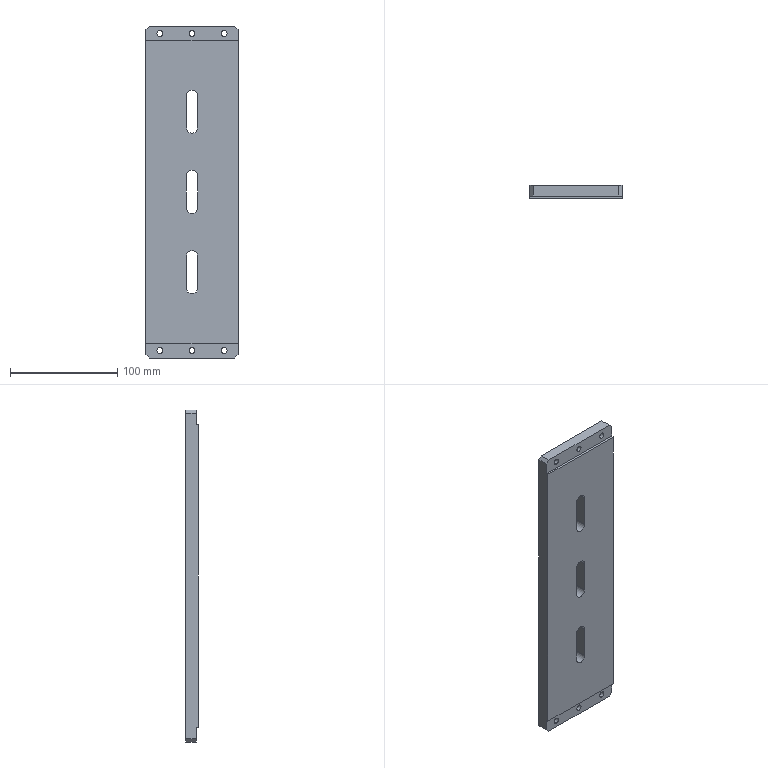Part | STEP file | 1 solid | 59 faces | box 86 x 12 x 310 mm | volume 297335 mm3 | cylinder 33 | plane 26 | commonest cylinder face diameters 5.5 x12 10 x12 10.4 x9